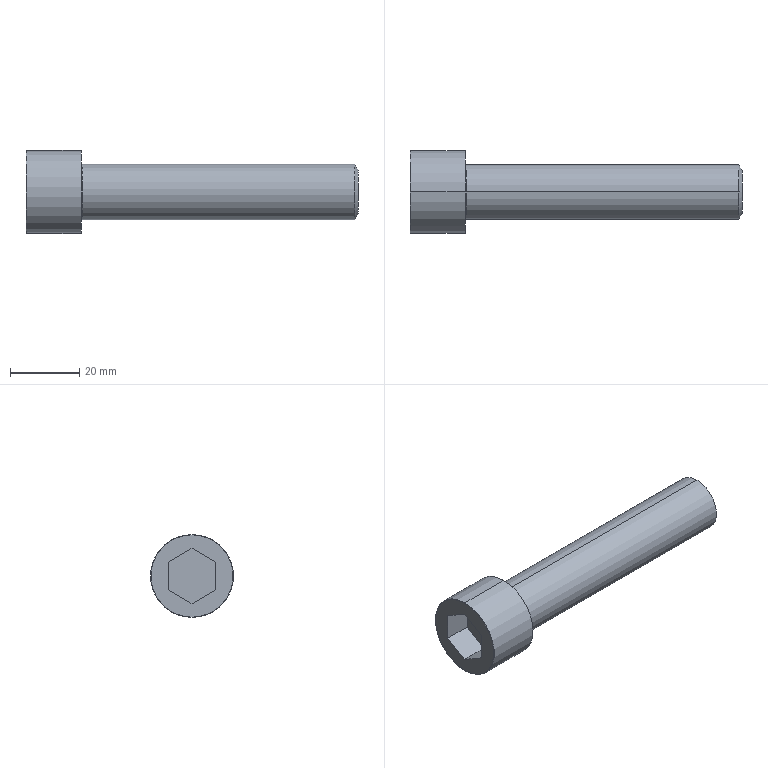Part | SolidWorks | features BlendCut 1, Cut 1, Fillet 1, LPattern 1, RevCut 1, Revolution 1 | 1 solid | 20 faces | box 96 x 24 x 24 mm | volume 21953 mm3 | plane 10 | torus 4 | cylinder 4 | cone 2 | commonest cylinder face diameters 16 x2 24 x2
STEP:
#1=CARTESIAN_POINT('',(0.,0.,11.9));
#2=VERTEX_POINT('',#1);
#3=CARTESIAN_POINT('',(0.,0.,-11.9));
#4=VERTEX_POINT('',#3);
#5=CARTESIAN_POINT('',(0.,0.,0.));
#6=DIRECTION('',(-1.,0.,0.));
#7=DIRECTION('',(0.,0.,-1.));
#8=AXIS2_PLACEMENT_3D('',#5,#6,#7);
#9=CIRCLE('',#8,11.9);
#10=EDGE_CURVE('',#2,#4,#9,.T.);
#11=ORIENTED_EDGE('',*,*,#10,.F.);
#12=CARTESIAN_POINT('',(0.1,0.,12.));
#13=VERTEX_POINT('',#12);
#14=CARTESIAN_POINT('',(0.1,0.,11.9));
#15=DIRECTION('',(0.,1.,0.));
#16=DIRECTION('',(0.,0.,1.));
#17=AXIS2_PLACEMENT_3D('',#14,#15,#16);
#18=CIRCLE('',#17,0.1);
#19=EDGE_CURVE('',#2,#13,#18,.T.);
#20=ORIENTED_EDGE('',*,*,#19,.T.);
#21=CARTESIAN_POINT('',(0.1,0.,-12.));
#22=VERTEX_POINT('',#21);
#23=CARTESIAN_POINT('',(0.1,0.,0.));
#24=DIRECTION('',(1.,0.,0.));
#25=DIRECTION('',(0.,0.,-1.));
#26=AXIS2_PLACEMENT_3D('',#23,#24,#25);
#27=CIRCLE('',#26,12.);
#28=EDGE_CURVE('',#22,#13,#27,.T.);
#29=ORIENTED_EDGE('',*,*,#28,.F.);
#30=CARTESIAN_POINT('',(0.1,0.,-11.9));
#31=DIRECTION('',(0.,-1.,0.));
#32=DIRECTION('',(0.,0.,-1.));
#33=AXIS2_PLACEMENT_3D('',#30,#31,#32);
#34=CIRCLE('',#33,0.1);
#35=EDGE_CURVE('',#4,#22,#34,.T.);
#36=ORIENTED_EDGE('',*,*,#35,.F.);
#37=EDGE_LOOP('',(#11,#20,#29,#36));
#38=FACE_OUTER_BOUND('',#37,.T.);
#39=CARTESIAN_POINT('',(0.1,0.,0.));
#40=DIRECTION('',(1.,0.,0.));
#41=DIRECTION('',(0.,0.,-1.));
#42=AXIS2_PLACEMENT_3D('',#39,#40,#41);
#43=TOROIDAL_SURFACE('',#42,11.9,0.1);
#44=ADVANCED_FACE('',(#38),#43,.T.);
#45=CARTESIAN_POINT('',(96.,0.,6.268));
#46=VERTEX_POINT('',#45);
#47=CARTESIAN_POINT('',(96.,0.,-6.268));
#48=VERTEX_POINT('',#47);
#49=CARTESIAN_POINT('',(96.,0.,0.));
#50=DIRECTION('',(-1.,0.,0.));
#51=DIRECTION('',(0.,0.,1.));
#52=AXIS2_PLACEMENT_3D('',#49,#50,#51);
#53=CIRCLE('',#52,6.268);
#54=EDGE_CURVE('',#46,#48,#53,.T.);
#55=ORIENTED_EDGE('',*,*,#54,.T.);
#56=CARTESIAN_POINT('',(95.,0.,-8.));
#57=VERTEX_POINT('',#56);
#58=CARTESIAN_POINT('',(95.,0.,-8.));
#59=DIRECTION('',(-0.5,0.,-0.866));
#60=VECTOR('',#59,1000.);
#61=LINE('',#58,#60);
#62=EDGE_CURVE('',#48,#57,#61,.T.);
#63=ORIENTED_EDGE('',*,*,#62,.T.);
#64=CARTESIAN_POINT('',(95.,0.,8.));
#65=VERTEX_POINT('',#64);
#66=CARTESIAN_POINT('',(95.,0.,0.));
#67=DIRECTION('',(-1.,0.,0.));
#68=DIRECTION('',(0.,0.,1.));
#69=AXIS2_PLACEMENT_3D('',#66,#67,#68);
#70=CIRCLE('',#69,8.);
#71=EDGE_CURVE('',#65,#57,#70,.T.);
#72=ORIENTED_EDGE('',*,*,#71,.F.);
#73=CARTESIAN_POINT('',(95.,0.,8.));
#74=DIRECTION('',(-0.5,0.,0.866));
#75=VECTOR('',#74,1000.);
#76=LINE('',#73,#75);
#77=EDGE_CURVE('',#46,#65,#76,.T.);
#78=ORIENTED_EDGE('',*,*,#77,.F.);
#79=EDGE_LOOP('',(#55,#63,#72,#78));
#80=FACE_OUTER_BOUND('',#79,.T.);
#81=CARTESIAN_POINT('',(95.,0.,0.));
#82=DIRECTION('',(-1.,0.,0.));
#83=DIRECTION('',(0.,0.,1.));
#84=AXIS2_PLACEMENT_3D('',#81,#82,#83);
#85=CONICAL_SURFACE('',#84,8.,1.047);
#86=ADVANCED_FACE('',(#80),#85,.T.);
#87=CARTESIAN_POINT('',(16.,0.,-8.2));
#88=VERTEX_POINT('',#87);
#89=CARTESIAN_POINT('',(16.,0.,8.2));
#90=VERTEX_POINT('',#89);
#91=CARTESIAN_POINT('',(16.,0.,0.));
#92=DIRECTION('',(-1.,0.,0.));
#93=DIRECTION('',(0.,0.,1.));
#94=AXIS2_PLACEMENT_3D('',#91,#92,#93);
#95=CIRCLE('',#94,8.2);
#96=EDGE_CURVE('',#88,#90,#95,.T.);
#97=ORIENTED_EDGE('',*,*,#96,.F.);
#98=CARTESIAN_POINT('',(16.2,0.,-8.));
#99=VERTEX_POINT('',#98);
#100=CARTESIAN_POINT('',(16.2,0.,-8.2));
#101=DIRECTION('',(0.,1.,0.));
#102=DIRECTION('',(0.,0.,1.));
#103=AXIS2_PLACEMENT_3D('',#100,#101,#102);
#104=CIRCLE('',#103,0.2);
#105=EDGE_CURVE('',#88,#99,#104,.T.);
#106=ORIENTED_EDGE('',*,*,#105,.T.);
#107=CARTESIAN_POINT('',(16.2,0.,8.));
#108=VERTEX_POINT('',#107);
#109=CARTESIAN_POINT('',(16.2,0.,0.));
#110=DIRECTION('',(-1.,0.,0.));
#111=DIRECTION('',(0.,0.,1.));
#112=AXIS2_PLACEMENT_3D('',#109,#110,#111);
#113=CIRCLE('',#112,8.);
#114=EDGE_CURVE('',#99,#108,#113,.T.);
#115=ORIENTED_EDGE('',*,*,#114,.T.);
#116=CARTESIAN_POINT('',(16.2,0.,8.2));
#117=DIRECTION('',(0.,-1.,0.));
#118=DIRECTION('',(0.,0.,-1.));
#119=AXIS2_PLACEMENT_3D('',#116,#117,#118);
#120=CIRCLE('',#119,0.2);
#121=EDGE_CURVE('',#90,#108,#120,.T.);
#122=ORIENTED_EDGE('',*,*,#121,.F.);
#123=EDGE_LOOP('',(#97,#106,#115,#122));
#124=FACE_OUTER_BOUND('',#123,.T.);
#125=CARTESIAN_POINT('',(16.2,0.,0.));
#126=DIRECTION('',(-1.,0.,0.));
#127=DIRECTION('',(0.,0.,1.));
#128=AXIS2_PLACEMENT_3D('',#125,#126,#127);
#129=TOROIDAL_SURFACE('',#128,8.2,0.2);
#130=ADVANCED_FACE('',(#124),#129,.F.);
#131=CARTESIAN_POINT('',(16.,0.,12.));
#132=VERTEX_POINT('',#131);
#133=CARTESIAN_POINT('',(16.,0.,-12.));
#134=VERTEX_POINT('',#133);
#135=CARTESIAN_POINT('',(16.,0.,0.));
#136=DIRECTION('',(-1.,0.,0.));
#137=DIRECTION('',(0.,0.,1.));
#138=AXIS2_PLACEMENT_3D('',#135,#136,#137);
#139=CIRCLE('',#138,12.);
#140=EDGE_CURVE('',#132,#134,#139,.T.);
#141=ORIENTED_EDGE('',*,*,#140,.T.);
#142=CARTESIAN_POINT('',(0.,0.,-12.));
#143=DIRECTION('',(-1.,0.,0.));
#144=VECTOR('',#143,1000.);
#145=LINE('',#142,#144);
#146=EDGE_CURVE('',#134,#22,#145,.T.);
#147=ORIENTED_EDGE('',*,*,#146,.T.);
#148=ORIENTED_EDGE('',*,*,#28,.T.);
#149=CARTESIAN_POINT('',(0.,0.,12.));
#150=DIRECTION('',(-1.,0.,0.));
#151=VECTOR('',#150,1000.);
#152=LINE('',#149,#151);
#153=EDGE_CURVE('',#132,#13,#152,.T.);
#154=ORIENTED_EDGE('',*,*,#153,.F.);
#155=EDGE_LOOP('',(#141,#147,#148,#154));
#156=FACE_OUTER_BOUND('',#155,.T.);
#157=CARTESIAN_POINT('',(0.,0.,0.));
#158=DIRECTION('',(-1.,0.,0.));
#159=DIRECTION('',(0.,0.,1.));
#160=AXIS2_PLACEMENT_3D('',#157,#158,#159);
#161=CYLINDRICAL_SURFACE('',#160,12.);
#162=ADVANCED_FACE('',(#156),#161,.T.);
#163=ORIENTED_EDGE('',*,*,#71,.T.);
#164=CARTESIAN_POINT('',(0.,0.,-8.));
#165=DIRECTION('',(-1.,0.,0.));
#166=VECTOR('',#165,1000.);
#167=LINE('',#164,#166);
#168=EDGE_CURVE('',#57,#99,#167,.T.);
#169=ORIENTED_EDGE('',*,*,#168,.T.);
#170=CARTESIAN_POINT('',(16.2,0.,0.));
#171=DIRECTION('',(-1.,0.,0.));
#172=DIRECTION('',(0.,0.,1.));
#173=AXIS2_PLACEMENT_3D('',#170,#171,#172);
#174=CIRCLE('',#173,8.);
#175=EDGE_CURVE('',#108,#99,#174,.T.);
#176=ORIENTED_EDGE('',*,*,#175,.F.);
#177=CARTESIAN_POINT('',(0.,0.,8.));
#178=DIRECTION('',(-1.,0.,0.));
#179=VECTOR('',#178,1000.);
#180=LINE('',#177,#179);
#181=EDGE_CURVE('',#65,#108,#180,.T.);
#182=ORIENTED_EDGE('',*,*,#181,.F.);
#183=EDGE_LOOP('',(#163,#169,#176,#182));
#184=FACE_OUTER_BOUND('',#183,.T.);
#185=CARTESIAN_POINT('',(0.,0.,0.));
#186=DIRECTION('',(-1.,0.,0.));
#187=DIRECTION('',(0.,0.,1.));
#188=AXIS2_PLACEMENT_3D('',#185,#186,#187);
#189=CYLINDRICAL_SURFACE('',#188,8.);
#190=ADVANCED_FACE('',(#184),#189,.T.);
#191=ORIENTED_EDGE('',*,*,#168,.F.);
#192=CARTESIAN_POINT('',(95.,0.,0.));
#193=DIRECTION('',(-1.,0.,0.));
#194=DIRECTION('',(0.,0.,1.));
#195=AXIS2_PLACEMENT_3D('',#192,#193,#194);
#196=CIRCLE('',#195,8.);
#197=EDGE_CURVE('',#57,#65,#196,.T.);
#198=ORIENTED_EDGE('',*,*,#197,.T.);
#199=ORIENTED_EDGE('',*,*,#181,.T.);
#200=ORIENTED_EDGE('',*,*,#114,.F.);
#201=EDGE_LOOP('',(#191,#198,#199,#200));
#202=FACE_OUTER_BOUND('',#201,.T.);
#203=CARTESIAN_POINT('',(0.,0.,0.));
#204=DIRECTION('',(-1.,0.,0.));
#205=DIRECTION('',(0.,0.,1.));
#206=AXIS2_PLACEMENT_3D('',#203,#204,#205);
#207=CYLINDRICAL_SURFACE('',#206,8.);
#208=ADVANCED_FACE('',(#202),#207,.T.);
#209=CARTESIAN_POINT('',(0.,0.,0.));
#210=DIRECTION('',(-1.,0.,0.));
#211=DIRECTION('',(0.,0.,-1.));
#212=AXIS2_PLACEMENT_3D('',#209,#210,#211);
#213=CIRCLE('',#212,11.9);
#214=EDGE_CURVE('',#4,#2,#213,.T.);
#215=ORIENTED_EDGE('',*,*,#214,.T.);
#216=ORIENTED_EDGE('',*,*,#10,.T.);
#217=EDGE_LOOP('',(#215,#216));
#218=FACE_OUTER_BOUND('',#217,.T.);
#219=CARTESIAN_POINT('',(0.,0.,8.));
#220=VERTEX_POINT('',#219);
#221=CARTESIAN_POINT('',(0.,6.928,4.));
#222=VERTEX_POINT('',#221);
#223=CARTESIAN_POINT('',(0.,0.,8.));
#224=DIRECTION('',(0.,0.866,-0.5));
#225=VECTOR('',#224,1000.);
#226=LINE('',#223,#225);
#227=EDGE_CURVE('',#220,#222,#226,.T.);
#228=ORIENTED_EDGE('',*,*,#227,.F.);
#229=CARTESIAN_POINT('',(0.,-6.928,4.));
#230=VERTEX_POINT('',#229);
#231=CARTESIAN_POINT('',(0.,-6.928,4.));
#232=DIRECTION('',(0.,0.866,0.5));
#233=VECTOR('',#232,1000.);
#234=LINE('',#231,#233);
#235=EDGE_CURVE('',#230,#220,#234,.T.);
#236=ORIENTED_EDGE('',*,*,#235,.F.);
#237=CARTESIAN_POINT('',(0.,-6.928,-4.));
#238=VERTEX_POINT('',#237);
#239=CARTESIAN_POINT('',(0.,-6.928,-4.));
#240=DIRECTION('',(0.,0.,1.));
#241=VECTOR('',#240,1000.);
#242=LINE('',#239,#241);
#243=EDGE_CURVE('',#238,#230,#242,.T.);
#244=ORIENTED_EDGE('',*,*,#243,.F.);
#245=CARTESIAN_POINT('',(0.,0.,-8.));
#246=VERTEX_POINT('',#245);
#247=CARTESIAN_POINT('',(0.,0.,-8.));
#248=DIRECTION('',(0.,-0.866,0.5));
#249=VECTOR('',#248,1000.);
#250=LINE('',#247,#249);
#251=EDGE_CURVE('',#246,#238,#250,.T.);
#252=ORIENTED_EDGE('',*,*,#251,.F.);
#253=CARTESIAN_POINT('',(0.,6.928,-4.));
#254=VERTEX_POINT('',#253);
#255=CARTESIAN_POINT('',(0.,6.928,-4.));
#256=DIRECTION('',(0.,-0.866,-0.5));
#257=VECTOR('',#256,1000.);
#258=LINE('',#255,#257);
#259=EDGE_CURVE('',#254,#246,#258,.T.);
#260=ORIENTED_EDGE('',*,*,#259,.F.);
#261=CARTESIAN_POINT('',(0.,6.928,4.));
#262=DIRECTION('',(0.,0.,-1.));
#263=VECTOR('',#262,1000.);
#264=LINE('',#261,#263);
#265=EDGE_CURVE('',#222,#254,#264,.T.);
#266=ORIENTED_EDGE('',*,*,#265,.F.);
#267=EDGE_LOOP('',(#228,#236,#244,#252,#260,#266));
#268=FACE_BOUND('',#267,.T.);
#269=CARTESIAN_POINT('',(0.,0.,0.));
#270=DIRECTION('',(1.,0.,0.));
#271=DIRECTION('',(0.,0.,-1.));
#272=AXIS2_PLACEMENT_3D('',#269,#270,#271);
#273=PLANE('',#272);
#274=ADVANCED_FACE('',(#218,#268),#273,.F.);
#275=ORIENTED_EDGE('',*,*,#146,.F.);
#276=CARTESIAN_POINT('',(16.,0.,0.));
#277=DIRECTION('',(-1.,0.,0.));
#278=DIRECTION('',(0.,0.,1.));
#279=AXIS2_PLACEMENT_3D('',#276,#277,#278);
#280=CIRCLE('',#279,12.);
#281=EDGE_CURVE('',#134,#132,#280,.T.);
#282=ORIENTED_EDGE('',*,*,#281,.T.);
#283=ORIENTED_EDGE('',*,*,#153,.T.);
#284=CARTESIAN_POINT('',(0.1,0.,0.));
#285=DIRECTION('',(1.,0.,0.));
#286=DIRECTION('',(0.,0.,-1.));
#287=AXIS2_PLACEMENT_3D('',#284,#285,#286);
#288=CIRCLE('',#287,12.);
#289=EDGE_CURVE('',#13,#22,#288,.T.);
#290=ORIENTED_EDGE('',*,*,#289,.T.);
#291=EDGE_LOOP('',(#275,#282,#283,#290));
#292=FACE_OUTER_BOUND('',#291,.T.);
#293=CARTESIAN_POINT('',(0.,0.,0.));
#294=DIRECTION('',(-1.,0.,0.));
#295=DIRECTION('',(0.,0.,1.));
#296=AXIS2_PLACEMENT_3D('',#293,#294,#295);
#297=CYLINDRICAL_SURFACE('',#296,12.);
#298=ADVANCED_FACE('',(#292),#297,.T.);
#299=ORIENTED_EDGE('',*,*,#140,.F.);
#300=ORIENTED_EDGE('',*,*,#281,.F.);
#301=EDGE_LOOP('',(#299,#300));
#302=FACE_OUTER_BOUND('',#301,.T.);
#303=CARTESIAN_POINT('',(16.,0.,0.));
#304=DIRECTION('',(-1.,0.,0.));
#305=DIRECTION('',(0.,0.,1.));
#306=AXIS2_PLACEMENT_3D('',#303,#304,#305);
#307=CIRCLE('',#306,8.2);
#308=EDGE_CURVE('',#90,#88,#307,.T.);
#309=ORIENTED_EDGE('',*,*,#308,.T.);
#310=ORIENTED_EDGE('',*,*,#96,.T.);
#311=EDGE_LOOP('',(#309,#310));
#312=FACE_BOUND('',#311,.T.);
#313=CARTESIAN_POINT('',(16.,12.,0.));
#314=DIRECTION('',(-1.,0.,0.));
#315=DIRECTION('',(0.,0.,1.));
#316=AXIS2_PLACEMENT_3D('',#313,#314,#315);
#317=PLANE('',#316);
#318=ADVANCED_FACE('',(#302,#312),#317,.F.);
#319=ORIENTED_EDGE('',*,*,#105,.F.);
#320=ORIENTED_EDGE('',*,*,#308,.F.);
#321=ORIENTED_EDGE('',*,*,#121,.T.);
#322=ORIENTED_EDGE('',*,*,#175,.T.);
#323=EDGE_LOOP('',(#319,#320,#321,#322));
#324=FACE_OUTER_BOUND('',#323,.T.);
#325=CARTESIAN_POINT('',(16.2,0.,0.));
#326=DIRECTION('',(-1.,0.,0.));
#327=DIRECTION('',(0.,0.,1.));
#328=AXIS2_PLACEMENT_3D('',#325,#326,#327);
#329=TOROIDAL_SURFACE('',#328,8.2,0.2);
#330=ADVANCED_FACE('',(#324),#329,.F.);
#331=ORIENTED_EDGE('',*,*,#235,.T.);
#332=CARTESIAN_POINT('',(8.,0.,8.));
#333=VERTEX_POINT('',#332);
#334=CARTESIAN_POINT('',(8.,0.,8.));
#335=DIRECTION('',(-1.,0.,0.));
#336=VECTOR('',#335,1000.);
#337=LINE('',#334,#336);
#338=EDGE_CURVE('',#333,#220,#337,.T.);
#339=ORIENTED_EDGE('',*,*,#338,.F.);
#340=CARTESIAN_POINT('',(8.,-6.928,4.));
#341=VERTEX_POINT('',#340);
#342=CARTESIAN_POINT('',(8.,-6.928,4.));
#343=DIRECTION('',(0.,0.866,0.5));
#344=VECTOR('',#343,1000.);
#345=LINE('',#342,#344);
#346=EDGE_CURVE('',#341,#333,#345,.T.);
#347=ORIENTED_EDGE('',*,*,#346,.F.);
#348=CARTESIAN_POINT('',(8.,-6.928,4.));
#349=DIRECTION('',(-1.,0.,0.));
#350=VECTOR('',#349,1000.);
#351=LINE('',#348,#350);
#352=EDGE_CURVE('',#341,#230,#351,.T.);
#353=ORIENTED_EDGE('',*,*,#352,.T.);
#354=EDGE_LOOP('',(#331,#339,#347,#353));
#355=FACE_OUTER_BOUND('',#354,.T.);
#356=CARTESIAN_POINT('',(8.,-6.928,4.));
#357=DIRECTION('',(0.,-0.5,0.866));
#358=DIRECTION('',(0.,-0.866,-0.5));
#359=AXIS2_PLACEMENT_3D('',#356,#357,#358);
#360=PLANE('',#359);
#361=ADVANCED_FACE('',(#355),#360,.F.);
#362=ORIENTED_EDGE('',*,*,#243,.T.);
#363=ORIENTED_EDGE('',*,*,#352,.F.);
#364=CARTESIAN_POINT('',(8.,-6.928,-4.));
#365=VERTEX_POINT('',#364);
#366=CARTESIAN_POINT('',(8.,-6.928,-4.));
#367=DIRECTION('',(0.,0.,1.));
#368=VECTOR('',#367,1000.);
#369=LINE('',#366,#368);
#370=EDGE_CURVE('',#365,#341,#369,.T.);
#371=ORIENTED_EDGE('',*,*,#370,.F.);
#372=CARTESIAN_POINT('',(8.,-6.928,-4.));
#373=DIRECTION('',(-1.,0.,0.));
#374=VECTOR('',#373,1000.);
#375=LINE('',#372,#374);
#376=EDGE_CURVE('',#365,#238,#375,.T.);
#377=ORIENTED_EDGE('',*,*,#376,.T.);
#378=EDGE_LOOP('',(#362,#363,#371,#377));
#379=FACE_OUTER_BOUND('',#378,.T.);
#380=CARTESIAN_POINT('',(8.,-6.928,-4.));
#381=DIRECTION('',(0.,-1.,0.));
#382=DIRECTION('',(0.,0.,-1.));
#383=AXIS2_PLACEMENT_3D('',#380,#381,#382);
#384=PLANE('',#383);
#385=ADVANCED_FACE('',(#379),#384,.F.);
#386=ORIENTED_EDGE('',*,*,#251,.T.);
#387=ORIENTED_EDGE('',*,*,#376,.F.);
#388=CARTESIAN_POINT('',(8.,0.,-8.));
#389=VERTEX_POINT('',#388);
#390=CARTESIAN_POINT('',(8.,0.,-8.));
#391=DIRECTION('',(0.,-0.866,0.5));
#392=VECTOR('',#391,1000.);
#393=LINE('',#390,#392);
#394=EDGE_CURVE('',#389,#365,#393,.T.);
#395=ORIENTED_EDGE('',*,*,#394,.F.);
#396=CARTESIAN_POINT('',(8.,0.,-8.));
#397=DIRECTION('',(-1.,0.,0.));
#398=VECTOR('',#397,1000.);
#399=LINE('',#396,#398);
#400=EDGE_CURVE('',#389,#246,#399,.T.);
#401=ORIENTED_EDGE('',*,*,#400,.T.);
#402=EDGE_LOOP('',(#386,#387,#395,#401));
#403=FACE_OUTER_BOUND('',#402,.T.);
#404=CARTESIAN_POINT('',(8.,0.,-8.));
#405=DIRECTION('',(0.,-0.5,-0.866));
#406=DIRECTION('',(0.,0.866,-0.5));
#407=AXIS2_PLACEMENT_3D('',#404,#405,#406);
#408=PLANE('',#407);
#409=ADVANCED_FACE('',(#403),#408,.F.);
#410=ORIENTED_EDGE('',*,*,#259,.T.);
#411=ORIENTED_EDGE('',*,*,#400,.F.);
#412=CARTESIAN_POINT('',(8.,6.928,-4.));
#413=VERTEX_POINT('',#412);
#414=CARTESIAN_POINT('',(8.,6.928,-4.));
#415=DIRECTION('',(0.,-0.866,-0.5));
#416=VECTOR('',#415,1000.);
#417=LINE('',#414,#416);
#418=EDGE_CURVE('',#413,#389,#417,.T.);
#419=ORIENTED_EDGE('',*,*,#418,.F.);
#420=CARTESIAN_POINT('',(8.,6.928,-4.));
#421=DIRECTION('',(-1.,0.,0.));
#422=VECTOR('',#421,1000.);
#423=LINE('',#420,#422);
#424=EDGE_CURVE('',#413,#254,#423,.T.);
#425=ORIENTED_EDGE('',*,*,#424,.T.);
#426=EDGE_LOOP('',(#410,#411,#419,#425));
#427=FACE_OUTER_BOUND('',#426,.T.);
#428=CARTESIAN_POINT('',(8.,6.928,-4.));
#429=DIRECTION('',(0.,0.5,-0.866));
#430=DIRECTION('',(0.,0.866,0.5));
#431=AXIS2_PLACEMENT_3D('',#428,#429,#430);
#432=PLANE('',#431);
#433=ADVANCED_FACE('',(#427),#432,.F.);
#434=ORIENTED_EDGE('',*,*,#265,.T.);
#435=ORIENTED_EDGE('',*,*,#424,.F.);
#436=CARTESIAN_POINT('',(8.,6.928,4.));
#437=VERTEX_POINT('',#436);
#438=CARTESIAN_POINT('',(8.,6.928,4.));
#439=DIRECTION('',(0.,0.,-1.));
#440=VECTOR('',#439,1000.);
#441=LINE('',#438,#440);
#442=EDGE_CURVE('',#437,#413,#441,.T.);
#443=ORIENTED_EDGE('',*,*,#442,.F.);
#444=CARTESIAN_POINT('',(8.,6.928,4.));
#445=DIRECTION('',(-1.,0.,0.));
#446=VECTOR('',#445,1000.);
#447=LINE('',#444,#446);
#448=EDGE_CURVE('',#437,#222,#447,.T.);
#449=ORIENTED_EDGE('',*,*,#448,.T.);
#450=EDGE_LOOP('',(#434,#435,#443,#449));
#451=FACE_OUTER_BOUND('',#450,.T.);
#452=CARTESIAN_POINT('',(8.,6.928,4.));
#453=DIRECTION('',(0.,1.,0.));
#454=DIRECTION('',(0.,0.,1.));
#455=AXIS2_PLACEMENT_3D('',#452,#453,#454);
#456=PLANE('',#455);
#457=ADVANCED_FACE('',(#451),#456,.F.);
#458=ORIENTED_EDGE('',*,*,#227,.T.);
#459=ORIENTED_EDGE('',*,*,#448,.F.);
#460=CARTESIAN_POINT('',(8.,0.,8.));
#461=DIRECTION('',(0.,0.866,-0.5));
#462=VECTOR('',#461,1000.);
#463=LINE('',#460,#462);
#464=EDGE_CURVE('',#333,#437,#463,.T.);
#465=ORIENTED_EDGE('',*,*,#464,.F.);
#466=ORIENTED_EDGE('',*,*,#338,.T.);
#467=EDGE_LOOP('',(#458,#459,#465,#466));
#468=FACE_OUTER_BOUND('',#467,.T.);
#469=CARTESIAN_POINT('',(8.,0.,8.));
#470=DIRECTION('',(0.,0.5,0.866));
#471=DIRECTION('',(0.,-0.866,0.5));
#472=AXIS2_PLACEMENT_3D('',#469,#470,#471);
#473=PLANE('',#472);
#474=ADVANCED_FACE('',(#468),#473,.F.);
#475=ORIENTED_EDGE('',*,*,#346,.T.);
#476=ORIENTED_EDGE('',*,*,#464,.T.);
#477=ORIENTED_EDGE('',*,*,#442,.T.);
#478=ORIENTED_EDGE('',*,*,#418,.T.);
#479=ORIENTED_EDGE('',*,*,#394,.T.);
#480=ORIENTED_EDGE('',*,*,#370,.T.);
#481=EDGE_LOOP('',(#475,#476,#477,#478,#479,#480));
#482=FACE_OUTER_BOUND('',#481,.T.);
#483=CARTESIAN_POINT('',(8.,-6.928,4.));
#484=DIRECTION('',(1.,0.,0.));
#485=DIRECTION('',(0.,0.,-1.));
#486=AXIS2_PLACEMENT_3D('',#483,#484,#485);
#487=PLANE('',#486);
#488=ADVANCED_FACE('',(#482),#487,.F.);
#489=ORIENTED_EDGE('',*,*,#62,.F.);
#490=CARTESIAN_POINT('',(96.,0.,0.));
#491=DIRECTION('',(-1.,0.,0.));
#492=DIRECTION('',(0.,0.,1.));
#493=AXIS2_PLACEMENT_3D('',#490,#491,#492);
#494=CIRCLE('',#493,6.268);
#495=EDGE_CURVE('',#48,#46,#494,.T.);
#496=ORIENTED_EDGE('',*,*,#495,.T.);
#497=ORIENTED_EDGE('',*,*,#77,.T.);
#498=ORIENTED_EDGE('',*,*,#197,.F.);
#499=EDGE_LOOP('',(#489,#496,#497,#498));
#500=FACE_OUTER_BOUND('',#499,.T.);
#501=CARTESIAN_POINT('',(95.,0.,0.));
#502=DIRECTION('',(-1.,0.,0.));
#503=DIRECTION('',(0.,0.,1.));
#504=AXIS2_PLACEMENT_3D('',#501,#502,#503);
#505=CONICAL_SURFACE('',#504,8.,1.047);
#506=ADVANCED_FACE('',(#500),#505,.T.);
#507=ORIENTED_EDGE('',*,*,#54,.F.);
#508=ORIENTED_EDGE('',*,*,#495,.F.);
#509=EDGE_LOOP('',(#507,#508));
#510=FACE_OUTER_BOUND('',#509,.T.);
#511=CARTESIAN_POINT('',(96.,8.,0.));
#512=DIRECTION('',(-1.,0.,0.));
#513=DIRECTION('',(0.,0.,1.));
#514=AXIS2_PLACEMENT_3D('',#511,#512,#513);
#515=PLANE('',#514);
#516=ADVANCED_FACE('',(#510),#515,.F.);
#517=ORIENTED_EDGE('',*,*,#19,.F.);
#518=ORIENTED_EDGE('',*,*,#214,.F.);
#519=ORIENTED_EDGE('',*,*,#35,.T.);
#520=ORIENTED_EDGE('',*,*,#289,.F.);
#521=EDGE_LOOP('',(#517,#518,#519,#520));
#522=FACE_OUTER_BOUND('',#521,.T.);
#523=CARTESIAN_POINT('',(0.1,0.,0.));
#524=DIRECTION('',(1.,0.,0.));
#525=DIRECTION('',(0.,0.,-1.));
#526=AXIS2_PLACEMENT_3D('',#523,#524,#525);
#527=TOROIDAL_SURFACE('',#526,11.9,0.1);
#528=ADVANCED_FACE('',(#522),#527,.T.);
#529=CLOSED_SHELL('',(#44,#86,#130,#162,#190,#208,#274,#298,#318,#330,#361,#385,#409,#433,#457,#474,#488,#506,#516,#528));
#530=MANIFOLD_SOLID_BREP('',#529);
#531=CARTESIAN_POINT('',(0.,0.,0.));
#532=DIRECTION('',(0.,0.,1.));
#533=DIRECTION('',(1.,0.,0.));
#534=AXIS2_PLACEMENT_3D('',#531,#532,#533);
#535=(LENGTH_UNIT()NAMED_UNIT(*)SI_UNIT(.MILLI.,.METRE.));
#536=UNCERTAINTY_MEASURE_WITH_UNIT(LENGTH_MEASURE(0.00001),#535,'','');
#537=(NAMED_UNIT(*)PLANE_ANGLE_UNIT()SI_UNIT($,.RADIAN.));
#538=(NAMED_UNIT(*)SI_UNIT($,.STERADIAN.)SOLID_ANGLE_UNIT());
#539=(GEOMETRIC_REPRESENTATION_CONTEXT(3)GLOBAL_UNCERTAINTY_ASSIGNED_CONTEXT((#536))GLOBAL_UNIT_ASSIGNED_CONTEXT((#535,#537,#538))REPRESENTATION_CONTEXT('',''));
#540=ADVANCED_BREP_SHAPE_REPRESENTATION('',(#530,#534),#539);